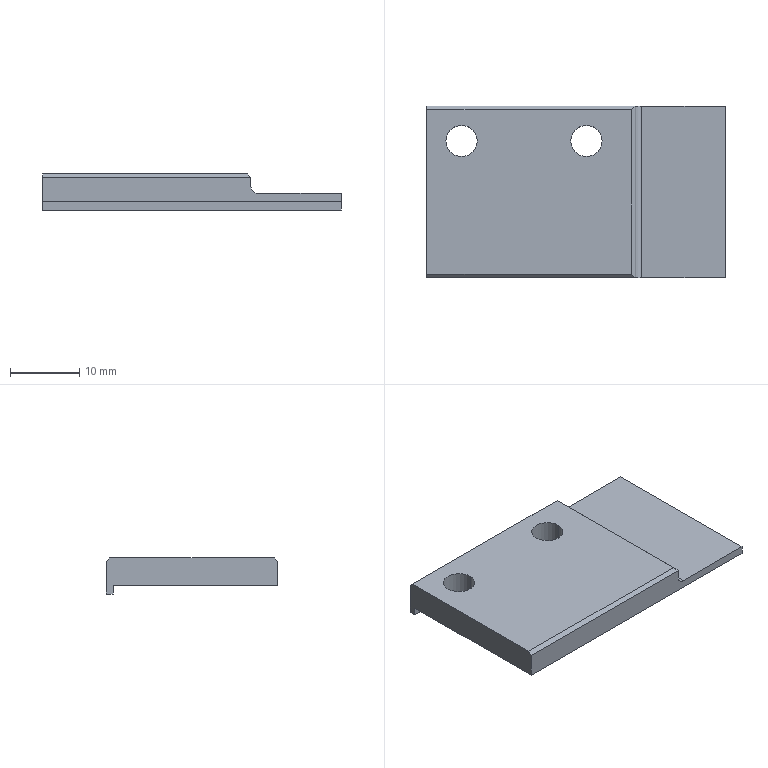Part | NX | 1 solid | 18 faces | box 43 x 24.7 x 5.2 mm | volume 3268 mm3 | plane 13 | cylinder 5 | commonest cylinder face diameters 4.5 x4 2 x1
STEP:
#1=CARTESIAN_POINT('',(0.,0.,-0.2));
#2=VERTEX_POINT('',#1);
#3=CARTESIAN_POINT('',(0.,-1.,-0.2));
#4=VERTEX_POINT('',#3);
#5=CARTESIAN_POINT('',(0.,0.,-0.2));
#6=DIRECTION('',(0.,-1.,0.));
#7=VECTOR('',#6,1000.);
#8=LINE('',#5,#7);
#9=EDGE_CURVE('',#2,#4,#8,.T.);
#10=ORIENTED_EDGE('',*,*,#9,.F.);
#11=CARTESIAN_POINT('',(43.,0.,-0.2));
#12=VERTEX_POINT('',#11);
#13=CARTESIAN_POINT('',(0.,0.,-0.2));
#14=DIRECTION('',(1.,0.,0.));
#15=VECTOR('',#14,1000.);
#16=LINE('',#13,#15);
#17=EDGE_CURVE('',#2,#12,#16,.T.);
#18=ORIENTED_EDGE('',*,*,#17,.T.);
#19=CARTESIAN_POINT('',(43.,-1.,-0.2));
#20=VERTEX_POINT('',#19);
#21=CARTESIAN_POINT('',(43.,0.,-0.2));
#22=DIRECTION('',(0.,1.,0.));
#23=VECTOR('',#22,1000.);
#24=LINE('',#21,#23);
#25=EDGE_CURVE('',#20,#12,#24,.T.);
#26=ORIENTED_EDGE('',*,*,#25,.F.);
#27=CARTESIAN_POINT('',(0.,-1.,-0.2));
#28=DIRECTION('',(-1.,0.,0.));
#29=VECTOR('',#28,1000.);
#30=LINE('',#27,#29);
#31=EDGE_CURVE('',#20,#4,#30,.T.);
#32=ORIENTED_EDGE('',*,*,#31,.T.);
#33=EDGE_LOOP('',(#10,#18,#26,#32));
#34=FACE_BOUND('',#33,.T.);
#35=CARTESIAN_POINT('',(0.,0.,-0.2));
#36=DIRECTION('',(0.,0.,1.));
#37=DIRECTION('',(1.,0.,0.));
#38=AXIS2_PLACEMENT_3D('',#35,#36,#37);
#39=PLANE('',#38);
#40=ADVANCED_FACE('',(#34),#39,.F.);
#41=ORIENTED_EDGE('',*,*,#9,.T.);
#42=CARTESIAN_POINT('',(0.,-1.,1.));
#43=VERTEX_POINT('',#42);
#44=CARTESIAN_POINT('',(0.,-1.,0.));
#45=DIRECTION('',(0.,0.,-1.));
#46=VECTOR('',#45,1000.);
#47=LINE('',#44,#46);
#48=EDGE_CURVE('',#43,#4,#47,.T.);
#49=ORIENTED_EDGE('',*,*,#48,.F.);
#50=CARTESIAN_POINT('',(0.,-24.7,1.));
#51=VERTEX_POINT('',#50);
#52=CARTESIAN_POINT('',(0.,0.,1.));
#53=DIRECTION('',(0.,-1.,0.));
#54=VECTOR('',#53,1000.);
#55=LINE('',#52,#54);
#56=EDGE_CURVE('',#43,#51,#55,.T.);
#57=ORIENTED_EDGE('',*,*,#56,.T.);
#58=CARTESIAN_POINT('',(0.,-24.7,4.5));
#59=VERTEX_POINT('',#58);
#60=CARTESIAN_POINT('',(0.,-24.7,0.));
#61=DIRECTION('',(0.,0.,-1.));
#62=VECTOR('',#61,1000.);
#63=LINE('',#60,#62);
#64=EDGE_CURVE('',#59,#51,#63,.T.);
#65=ORIENTED_EDGE('',*,*,#64,.F.);
#66=CARTESIAN_POINT('',(0.,-24.2,5.));
#67=VERTEX_POINT('',#66);
#68=CARTESIAN_POINT('',(0.,-29.2,0.));
#69=DIRECTION('',(0.,0.7071,0.7071));
#70=VECTOR('',#69,1000.);
#71=LINE('',#68,#70);
#72=EDGE_CURVE('',#59,#67,#71,.T.);
#73=ORIENTED_EDGE('',*,*,#72,.T.);
#74=CARTESIAN_POINT('',(0.,-0.5,5.));
#75=VERTEX_POINT('',#74);
#76=CARTESIAN_POINT('',(0.,0.,5.));
#77=DIRECTION('',(0.,-1.,0.));
#78=VECTOR('',#77,1000.);
#79=LINE('',#76,#78);
#80=EDGE_CURVE('',#75,#67,#79,.T.);
#81=ORIENTED_EDGE('',*,*,#80,.F.);
#82=CARTESIAN_POINT('',(0.,0.,4.5));
#83=VERTEX_POINT('',#82);
#84=CARTESIAN_POINT('',(0.,4.5,0.));
#85=DIRECTION('',(0.,-0.7071,0.7071));
#86=VECTOR('',#85,1000.);
#87=LINE('',#84,#86);
#88=EDGE_CURVE('',#83,#75,#87,.T.);
#89=ORIENTED_EDGE('',*,*,#88,.F.);
#90=CARTESIAN_POINT('',(0.,0.,0.));
#91=DIRECTION('',(0.,0.,1.));
#92=VECTOR('',#91,1000.);
#93=LINE('',#90,#92);
#94=EDGE_CURVE('',#2,#83,#93,.T.);
#95=ORIENTED_EDGE('',*,*,#94,.F.);
#96=EDGE_LOOP('',(#41,#49,#57,#65,#73,#81,#89,#95));
#97=FACE_BOUND('',#96,.T.);
#98=CARTESIAN_POINT('',(0.,0.,0.));
#99=DIRECTION('',(-1.,0.,0.));
#100=DIRECTION('',(0.,0.,1.));
#101=AXIS2_PLACEMENT_3D('',#98,#99,#100);
#102=PLANE('',#101);
#103=ADVANCED_FACE('',(#97),#102,.T.);
#104=CARTESIAN_POINT('',(31.,0.,2.2));
#105=VERTEX_POINT('',#104);
#106=CARTESIAN_POINT('',(43.,0.,2.2));
#107=VERTEX_POINT('',#106);
#108=CARTESIAN_POINT('',(0.,0.,2.2));
#109=DIRECTION('',(1.,0.,0.));
#110=VECTOR('',#109,1000.);
#111=LINE('',#108,#110);
#112=EDGE_CURVE('',#105,#107,#111,.T.);
#113=ORIENTED_EDGE('',*,*,#112,.T.);
#114=CARTESIAN_POINT('',(43.,0.,0.));
#115=DIRECTION('',(0.,0.,-1.));
#116=VECTOR('',#115,1000.);
#117=LINE('',#114,#116);
#118=EDGE_CURVE('',#107,#12,#117,.T.);
#119=ORIENTED_EDGE('',*,*,#118,.T.);
#120=ORIENTED_EDGE('',*,*,#17,.F.);
#121=ORIENTED_EDGE('',*,*,#94,.T.);
#122=CARTESIAN_POINT('',(30.,0.,4.5));
#123=VERTEX_POINT('',#122);
#124=CARTESIAN_POINT('',(0.,0.,4.5));
#125=DIRECTION('',(1.,0.,0.));
#126=VECTOR('',#125,1000.);
#127=LINE('',#124,#126);
#128=EDGE_CURVE('',#83,#123,#127,.T.);
#129=ORIENTED_EDGE('',*,*,#128,.T.);
#130=CARTESIAN_POINT('',(30.,0.,3.2));
#131=VERTEX_POINT('',#130);
#132=CARTESIAN_POINT('',(30.,0.,0.));
#133=DIRECTION('',(0.,0.,1.));
#134=VECTOR('',#133,1000.);
#135=LINE('',#132,#134);
#136=EDGE_CURVE('',#131,#123,#135,.T.);
#137=ORIENTED_EDGE('',*,*,#136,.F.);
#138=CARTESIAN_POINT('',(31.,0.,3.2));
#139=DIRECTION('',(0.,1.,0.));
#140=DIRECTION('',(1.,0.,0.));
#141=AXIS2_PLACEMENT_3D('',#138,#139,#140);
#142=CIRCLE('',#141,1.);
#143=EDGE_CURVE('',#105,#131,#142,.T.);
#144=ORIENTED_EDGE('',*,*,#143,.F.);
#145=EDGE_LOOP('',(#113,#119,#120,#121,#129,#137,#144));
#146=FACE_BOUND('',#145,.T.);
#147=CARTESIAN_POINT('',(43.,0.,0.));
#148=DIRECTION('',(0.,1.,0.));
#149=DIRECTION('',(1.,0.,0.));
#150=AXIS2_PLACEMENT_3D('',#147,#148,#149);
#151=PLANE('',#150);
#152=ADVANCED_FACE('',(#146),#151,.T.);
#153=CARTESIAN_POINT('',(31.,-24.7,2.2));
#154=VERTEX_POINT('',#153);
#155=CARTESIAN_POINT('',(31.,0.,2.2));
#156=DIRECTION('',(0.,1.,0.));
#157=VECTOR('',#156,1000.);
#158=LINE('',#155,#157);
#159=EDGE_CURVE('',#154,#105,#158,.T.);
#160=ORIENTED_EDGE('',*,*,#159,.F.);
#161=CARTESIAN_POINT('',(43.,-24.7,2.2));
#162=VERTEX_POINT('',#161);
#163=CARTESIAN_POINT('',(0.,-24.7,2.2));
#164=DIRECTION('',(-1.,0.,0.));
#165=VECTOR('',#164,1000.);
#166=LINE('',#163,#165);
#167=EDGE_CURVE('',#162,#154,#166,.T.);
#168=ORIENTED_EDGE('',*,*,#167,.F.);
#169=CARTESIAN_POINT('',(43.,0.,2.2));
#170=DIRECTION('',(0.,-1.,0.));
#171=VECTOR('',#170,1000.);
#172=LINE('',#169,#171);
#173=EDGE_CURVE('',#107,#162,#172,.T.);
#174=ORIENTED_EDGE('',*,*,#173,.F.);
#175=ORIENTED_EDGE('',*,*,#112,.F.);
#176=EDGE_LOOP('',(#160,#168,#174,#175));
#177=FACE_BOUND('',#176,.T.);
#178=CARTESIAN_POINT('',(0.,0.,2.2));
#179=DIRECTION('',(0.,0.,1.));
#180=DIRECTION('',(1.,0.,0.));
#181=AXIS2_PLACEMENT_3D('',#178,#179,#180);
#182=PLANE('',#181);
#183=ADVANCED_FACE('',(#177),#182,.T.);
#184=CARTESIAN_POINT('',(30.,-24.7,4.5));
#185=VERTEX_POINT('',#184);
#186=CARTESIAN_POINT('',(30.,0.,4.5));
#187=DIRECTION('',(0.,1.,0.));
#188=VECTOR('',#187,1000.);
#189=LINE('',#186,#188);
#190=EDGE_CURVE('',#185,#123,#189,.T.);
#191=ORIENTED_EDGE('',*,*,#190,.T.);
#192=CARTESIAN_POINT('',(29.5,-0.5,5.));
#193=VERTEX_POINT('',#192);
#194=CARTESIAN_POINT('',(34.5,4.5,0.));
#195=DIRECTION('',(0.5774,0.5774,-0.5774));
#196=VECTOR('',#195,1000.);
#197=LINE('',#194,#196);
#198=EDGE_CURVE('',#193,#123,#197,.T.);
#199=ORIENTED_EDGE('',*,*,#198,.F.);
#200=CARTESIAN_POINT('',(29.5,-24.2,5.));
#201=VERTEX_POINT('',#200);
#202=CARTESIAN_POINT('',(29.5,0.,5.));
#203=DIRECTION('',(0.,1.,0.));
#204=VECTOR('',#203,1000.);
#205=LINE('',#202,#204);
#206=EDGE_CURVE('',#201,#193,#205,.T.);
#207=ORIENTED_EDGE('',*,*,#206,.F.);
#208=CARTESIAN_POINT('',(34.5,-29.2,0.));
#209=DIRECTION('',(0.5774,-0.5774,-0.5774));
#210=VECTOR('',#209,1000.);
#211=LINE('',#208,#210);
#212=EDGE_CURVE('',#201,#185,#211,.T.);
#213=ORIENTED_EDGE('',*,*,#212,.T.);
#214=EDGE_LOOP('',(#191,#199,#207,#213));
#215=FACE_BOUND('',#214,.T.);
#216=CARTESIAN_POINT('',(29.75,-12.35,4.75));
#217=DIRECTION('',(-0.7071,0.,-0.7071));
#218=DIRECTION('',(-0.7071,0.,0.7071));
#219=AXIS2_PLACEMENT_3D('',#216,#217,#218);
#220=PLANE('',#219);
#221=ADVANCED_FACE('',(#215),#220,.F.);
#222=CARTESIAN_POINT('',(30.,-24.7,3.2));
#223=VERTEX_POINT('',#222);
#224=CARTESIAN_POINT('',(30.,-24.7,0.));
#225=DIRECTION('',(0.,0.,-1.));
#226=VECTOR('',#225,1000.);
#227=LINE('',#224,#226);
#228=EDGE_CURVE('',#185,#223,#227,.T.);
#229=ORIENTED_EDGE('',*,*,#228,.F.);
#230=CARTESIAN_POINT('',(0.,-24.7,4.5));
#231=DIRECTION('',(1.,0.,0.));
#232=VECTOR('',#231,1000.);
#233=LINE('',#230,#232);
#234=EDGE_CURVE('',#59,#185,#233,.T.);
#235=ORIENTED_EDGE('',*,*,#234,.F.);
#236=ORIENTED_EDGE('',*,*,#64,.T.);
#237=CARTESIAN_POINT('',(43.,-24.7,1.));
#238=VERTEX_POINT('',#237);
#239=CARTESIAN_POINT('',(0.,-24.7,1.));
#240=DIRECTION('',(-1.,0.,0.));
#241=VECTOR('',#240,1000.);
#242=LINE('',#239,#241);
#243=EDGE_CURVE('',#238,#51,#242,.T.);
#244=ORIENTED_EDGE('',*,*,#243,.F.);
#245=CARTESIAN_POINT('',(43.,-24.7,0.));
#246=DIRECTION('',(0.,0.,1.));
#247=VECTOR('',#246,1000.);
#248=LINE('',#245,#247);
#249=EDGE_CURVE('',#238,#162,#248,.T.);
#250=ORIENTED_EDGE('',*,*,#249,.T.);
#251=ORIENTED_EDGE('',*,*,#167,.T.);
#252=CARTESIAN_POINT('',(31.,-24.7,3.2));
#253=DIRECTION('',(0.,1.,0.));
#254=DIRECTION('',(1.,0.,0.));
#255=AXIS2_PLACEMENT_3D('',#252,#253,#254);
#256=CIRCLE('',#255,1.);
#257=EDGE_CURVE('',#154,#223,#256,.T.);
#258=ORIENTED_EDGE('',*,*,#257,.T.);
#259=EDGE_LOOP('',(#229,#235,#236,#244,#250,#251,#258));
#260=FACE_BOUND('',#259,.T.);
#261=CARTESIAN_POINT('',(0.,-24.7,0.));
#262=DIRECTION('',(0.,-1.,0.));
#263=DIRECTION('',(0.,0.,-1.));
#264=AXIS2_PLACEMENT_3D('',#261,#262,#263);
#265=PLANE('',#264);
#266=ADVANCED_FACE('',(#260),#265,.T.);
#267=CARTESIAN_POINT('',(30.,0.,3.2));
#268=DIRECTION('',(0.,1.,0.));
#269=VECTOR('',#268,1000.);
#270=LINE('',#267,#269);
#271=EDGE_CURVE('',#223,#131,#270,.T.);
#272=ORIENTED_EDGE('',*,*,#271,.T.);
#273=ORIENTED_EDGE('',*,*,#136,.T.);
#274=ORIENTED_EDGE('',*,*,#190,.F.);
#275=ORIENTED_EDGE('',*,*,#228,.T.);
#276=EDGE_LOOP('',(#272,#273,#274,#275));
#277=FACE_BOUND('',#276,.T.);
#278=CARTESIAN_POINT('',(30.,0.,5.));
#279=DIRECTION('',(-1.,0.,0.));
#280=DIRECTION('',(0.,0.,1.));
#281=AXIS2_PLACEMENT_3D('',#278,#279,#280);
#282=PLANE('',#281);
#283=ADVANCED_FACE('',(#277),#282,.F.);
#284=ORIENTED_EDGE('',*,*,#206,.T.);
#285=CARTESIAN_POINT('',(0.,-0.5,5.));
#286=DIRECTION('',(1.,0.,0.));
#287=VECTOR('',#286,1000.);
#288=LINE('',#285,#287);
#289=EDGE_CURVE('',#75,#193,#288,.T.);
#290=ORIENTED_EDGE('',*,*,#289,.F.);
#291=ORIENTED_EDGE('',*,*,#80,.T.);
#292=CARTESIAN_POINT('',(0.,-24.2,5.));
#293=DIRECTION('',(1.,0.,0.));
#294=VECTOR('',#293,1000.);
#295=LINE('',#292,#294);
#296=EDGE_CURVE('',#67,#201,#295,.T.);
#297=ORIENTED_EDGE('',*,*,#296,.T.);
#298=EDGE_LOOP('',(#284,#290,#291,#297));
#299=FACE_BOUND('',#298,.T.);
#300=CARTESIAN_POINT('',(20.75,-5.,5.));
#301=VERTEX_POINT('',#300);
#302=CARTESIAN_POINT('',(25.25,-5.,5.));
#303=VERTEX_POINT('',#302);
#304=CARTESIAN_POINT('',(23.,-5.,5.));
#305=DIRECTION('',(0.,0.,-1.));
#306=DIRECTION('',(-1.,0.,0.));
#307=AXIS2_PLACEMENT_3D('',#304,#305,#306);
#308=CIRCLE('',#307,2.25);
#309=EDGE_CURVE('',#301,#303,#308,.T.);
#310=ORIENTED_EDGE('',*,*,#309,.T.);
#311=CARTESIAN_POINT('',(23.,-5.,5.));
#312=DIRECTION('',(0.,0.,-1.));
#313=DIRECTION('',(-1.,0.,0.));
#314=AXIS2_PLACEMENT_3D('',#311,#312,#313);
#315=CIRCLE('',#314,2.25);
#316=EDGE_CURVE('',#303,#301,#315,.T.);
#317=ORIENTED_EDGE('',*,*,#316,.T.);
#318=EDGE_LOOP('',(#310,#317));
#319=FACE_BOUND('',#318,.T.);
#320=CARTESIAN_POINT('',(7.25,-5.,5.));
#321=VERTEX_POINT('',#320);
#322=CARTESIAN_POINT('',(2.75,-5.,5.));
#323=VERTEX_POINT('',#322);
#324=CARTESIAN_POINT('',(5.,-5.,5.));
#325=DIRECTION('',(0.,0.,-1.));
#326=DIRECTION('',(-1.,0.,0.));
#327=AXIS2_PLACEMENT_3D('',#324,#325,#326);
#328=CIRCLE('',#327,2.25);
#329=EDGE_CURVE('',#321,#323,#328,.T.);
#330=ORIENTED_EDGE('',*,*,#329,.T.);
#331=CARTESIAN_POINT('',(5.,-5.,5.));
#332=DIRECTION('',(0.,0.,-1.));
#333=DIRECTION('',(-1.,0.,0.));
#334=AXIS2_PLACEMENT_3D('',#331,#332,#333);
#335=CIRCLE('',#334,2.25);
#336=EDGE_CURVE('',#323,#321,#335,.T.);
#337=ORIENTED_EDGE('',*,*,#336,.T.);
#338=EDGE_LOOP('',(#330,#337));
#339=FACE_BOUND('',#338,.T.);
#340=CARTESIAN_POINT('',(0.,0.,5.));
#341=DIRECTION('',(0.,0.,1.));
#342=DIRECTION('',(1.,0.,0.));
#343=AXIS2_PLACEMENT_3D('',#340,#341,#342);
#344=PLANE('',#343);
#345=ADVANCED_FACE('',(#299,#319,#339),#344,.T.);
#346=CARTESIAN_POINT('',(20.75,-5.,1.));
#347=VERTEX_POINT('',#346);
#348=CARTESIAN_POINT('',(25.25,-5.,1.));
#349=VERTEX_POINT('',#348);
#350=CARTESIAN_POINT('',(23.,-5.,1.));
#351=DIRECTION('',(0.,0.,-1.));
#352=DIRECTION('',(-1.,0.,0.));
#353=AXIS2_PLACEMENT_3D('',#350,#351,#352);
#354=CIRCLE('',#353,2.25);
#355=EDGE_CURVE('',#347,#349,#354,.T.);
#356=ORIENTED_EDGE('',*,*,#355,.T.);
#357=CARTESIAN_POINT('',(25.25,-5.,5.));
#358=DIRECTION('',(0.,0.,-1.));
#359=VECTOR('',#358,1000.);
#360=LINE('',#357,#359);
#361=EDGE_CURVE('',#349,#303,#360,.F.);
#362=ORIENTED_EDGE('',*,*,#361,.T.);
#363=ORIENTED_EDGE('',*,*,#309,.F.);
#364=CARTESIAN_POINT('',(20.75,-5.,5.));
#365=DIRECTION('',(0.,0.,-1.));
#366=VECTOR('',#365,1000.);
#367=LINE('',#364,#366);
#368=EDGE_CURVE('',#347,#301,#367,.F.);
#369=ORIENTED_EDGE('',*,*,#368,.F.);
#370=EDGE_LOOP('',(#356,#362,#363,#369));
#371=FACE_BOUND('',#370,.T.);
#372=CARTESIAN_POINT('',(23.,-5.,5.));
#373=DIRECTION('',(0.,0.,-1.));
#374=DIRECTION('',(-1.,0.,0.));
#375=AXIS2_PLACEMENT_3D('',#372,#373,#374);
#376=CYLINDRICAL_SURFACE('',#375,2.25);
#377=ADVANCED_FACE('',(#371),#376,.F.);
#378=ORIENTED_EDGE('',*,*,#329,.F.);
#379=CARTESIAN_POINT('',(7.25,-5.,1.));
#380=VERTEX_POINT('',#379);
#381=CARTESIAN_POINT('',(7.25,-5.,5.));
#382=DIRECTION('',(0.,0.,-1.));
#383=VECTOR('',#382,1000.);
#384=LINE('',#381,#383);
#385=EDGE_CURVE('',#321,#380,#384,.T.);
#386=ORIENTED_EDGE('',*,*,#385,.T.);
#387=CARTESIAN_POINT('',(2.75,-5.,1.));
#388=VERTEX_POINT('',#387);
#389=CARTESIAN_POINT('',(5.,-5.,1.));
#390=DIRECTION('',(0.,0.,-1.));
#391=DIRECTION('',(-1.,0.,0.));
#392=AXIS2_PLACEMENT_3D('',#389,#390,#391);
#393=CIRCLE('',#392,2.25);
#394=EDGE_CURVE('',#380,#388,#393,.T.);
#395=ORIENTED_EDGE('',*,*,#394,.T.);
#396=CARTESIAN_POINT('',(2.75,-5.,5.));
#397=DIRECTION('',(0.,0.,-1.));
#398=VECTOR('',#397,1000.);
#399=LINE('',#396,#398);
#400=EDGE_CURVE('',#323,#388,#399,.T.);
#401=ORIENTED_EDGE('',*,*,#400,.F.);
#402=EDGE_LOOP('',(#378,#386,#395,#401));
#403=FACE_BOUND('',#402,.T.);
#404=CARTESIAN_POINT('',(5.,-5.,5.));
#405=DIRECTION('',(0.,0.,-1.));
#406=DIRECTION('',(-1.,0.,0.));
#407=AXIS2_PLACEMENT_3D('',#404,#405,#406);
#408=CYLINDRICAL_SURFACE('',#407,2.25);
#409=ADVANCED_FACE('',(#403),#408,.F.);
#410=ORIENTED_EDGE('',*,*,#56,.F.);
#411=CARTESIAN_POINT('',(43.,-1.,1.));
#412=VERTEX_POINT('',#411);
#413=CARTESIAN_POINT('',(0.,-1.,1.));
#414=DIRECTION('',(-1.,0.,0.));
#415=VECTOR('',#414,1000.);
#416=LINE('',#413,#415);
#417=EDGE_CURVE('',#412,#43,#416,.T.);
#418=ORIENTED_EDGE('',*,*,#417,.F.);
#419=CARTESIAN_POINT('',(43.,0.,1.));
#420=DIRECTION('',(0.,1.,0.));
#421=VECTOR('',#420,1000.);
#422=LINE('',#419,#421);
#423=EDGE_CURVE('',#238,#412,#422,.T.);
#424=ORIENTED_EDGE('',*,*,#423,.F.);
#425=ORIENTED_EDGE('',*,*,#243,.T.);
#426=EDGE_LOOP('',(#410,#418,#424,#425));
#427=FACE_BOUND('',#426,.T.);
#428=ORIENTED_EDGE('',*,*,#355,.F.);
#429=CARTESIAN_POINT('',(23.,-5.,1.));
#430=DIRECTION('',(0.,0.,-1.));
#431=DIRECTION('',(-1.,0.,0.));
#432=AXIS2_PLACEMENT_3D('',#429,#430,#431);
#433=CIRCLE('',#432,2.25);
#434=EDGE_CURVE('',#349,#347,#433,.T.);
#435=ORIENTED_EDGE('',*,*,#434,.F.);
#436=EDGE_LOOP('',(#428,#435));
#437=FACE_BOUND('',#436,.T.);
#438=CARTESIAN_POINT('',(5.,-5.,1.));
#439=DIRECTION('',(0.,0.,-1.));
#440=DIRECTION('',(-1.,0.,0.));
#441=AXIS2_PLACEMENT_3D('',#438,#439,#440);
#442=CIRCLE('',#441,2.25);
#443=EDGE_CURVE('',#388,#380,#442,.T.);
#444=ORIENTED_EDGE('',*,*,#443,.F.);
#445=ORIENTED_EDGE('',*,*,#394,.F.);
#446=EDGE_LOOP('',(#444,#445));
#447=FACE_BOUND('',#446,.T.);
#448=CARTESIAN_POINT('',(0.,-26.7,1.));
#449=DIRECTION('',(0.,0.,1.));
#450=DIRECTION('',(1.,0.,0.));
#451=AXIS2_PLACEMENT_3D('',#448,#449,#450);
#452=PLANE('',#451);
#453=ADVANCED_FACE('',(#427,#437,#447),#452,.F.);
#454=ORIENTED_EDGE('',*,*,#173,.T.);
#455=ORIENTED_EDGE('',*,*,#249,.F.);
#456=ORIENTED_EDGE('',*,*,#423,.T.);
#457=CARTESIAN_POINT('',(43.,-1.,0.));
#458=DIRECTION('',(0.,0.,-1.));
#459=VECTOR('',#458,1000.);
#460=LINE('',#457,#459);
#461=EDGE_CURVE('',#412,#20,#460,.T.);
#462=ORIENTED_EDGE('',*,*,#461,.T.);
#463=ORIENTED_EDGE('',*,*,#25,.T.);
#464=ORIENTED_EDGE('',*,*,#118,.F.);
#465=EDGE_LOOP('',(#454,#455,#456,#462,#463,#464));
#466=FACE_BOUND('',#465,.T.);
#467=CARTESIAN_POINT('',(43.,-26.7,0.));
#468=DIRECTION('',(1.,0.,0.));
#469=DIRECTION('',(0.,1.,0.));
#470=AXIS2_PLACEMENT_3D('',#467,#468,#469);
#471=PLANE('',#470);
#472=ADVANCED_FACE('',(#466),#471,.T.);
#473=ORIENTED_EDGE('',*,*,#31,.F.);
#474=ORIENTED_EDGE('',*,*,#461,.F.);
#475=ORIENTED_EDGE('',*,*,#417,.T.);
#476=ORIENTED_EDGE('',*,*,#48,.T.);
#477=EDGE_LOOP('',(#473,#474,#475,#476));
#478=FACE_BOUND('',#477,.T.);
#479=CARTESIAN_POINT('',(0.,-1.,1.));
#480=DIRECTION('',(0.,1.,0.));
#481=DIRECTION('',(1.,0.,0.));
#482=AXIS2_PLACEMENT_3D('',#479,#480,#481);
#483=PLANE('',#482);
#484=ADVANCED_FACE('',(#478),#483,.F.);
#485=ORIENTED_EDGE('',*,*,#128,.F.);
#486=ORIENTED_EDGE('',*,*,#88,.T.);
#487=ORIENTED_EDGE('',*,*,#289,.T.);
#488=ORIENTED_EDGE('',*,*,#198,.T.);
#489=EDGE_LOOP('',(#485,#486,#487,#488));
#490=FACE_BOUND('',#489,.T.);
#491=CARTESIAN_POINT('',(15.,-0.25,4.75));
#492=DIRECTION('',(0.,0.7071,0.7071));
#493=DIRECTION('',(1.,0.,0.));
#494=AXIS2_PLACEMENT_3D('',#491,#492,#493);
#495=PLANE('',#494);
#496=ADVANCED_FACE('',(#490),#495,.T.);
#497=ORIENTED_EDGE('',*,*,#234,.T.);
#498=ORIENTED_EDGE('',*,*,#212,.F.);
#499=ORIENTED_EDGE('',*,*,#296,.F.);
#500=ORIENTED_EDGE('',*,*,#72,.F.);
#501=EDGE_LOOP('',(#497,#498,#499,#500));
#502=FACE_BOUND('',#501,.T.);
#503=CARTESIAN_POINT('',(15.,-24.45,4.75));
#504=DIRECTION('',(0.,0.7071,-0.7071));
#505=DIRECTION('',(-1.,0.,0.));
#506=AXIS2_PLACEMENT_3D('',#503,#504,#505);
#507=PLANE('',#506);
#508=ADVANCED_FACE('',(#502),#507,.F.);
#509=ORIENTED_EDGE('',*,*,#159,.T.);
#510=ORIENTED_EDGE('',*,*,#143,.T.);
#511=ORIENTED_EDGE('',*,*,#271,.F.);
#512=ORIENTED_EDGE('',*,*,#257,.F.);
#513=EDGE_LOOP('',(#509,#510,#511,#512));
#514=FACE_BOUND('',#513,.T.);
#515=CARTESIAN_POINT('',(31.,0.,3.2));
#516=DIRECTION('',(0.,1.,0.));
#517=DIRECTION('',(1.,0.,0.));
#518=AXIS2_PLACEMENT_3D('',#515,#516,#517);
#519=CYLINDRICAL_SURFACE('',#518,1.);
#520=ADVANCED_FACE('',(#514),#519,.F.);
#521=ORIENTED_EDGE('',*,*,#368,.T.);
#522=ORIENTED_EDGE('',*,*,#316,.F.);
#523=ORIENTED_EDGE('',*,*,#361,.F.);
#524=ORIENTED_EDGE('',*,*,#434,.T.);
#525=EDGE_LOOP('',(#521,#522,#523,#524));
#526=FACE_BOUND('',#525,.T.);
#527=CARTESIAN_POINT('',(23.,-5.,5.));
#528=DIRECTION('',(0.,0.,-1.));
#529=DIRECTION('',(-1.,0.,0.));
#530=AXIS2_PLACEMENT_3D('',#527,#528,#529);
#531=CYLINDRICAL_SURFACE('',#530,2.25);
#532=ADVANCED_FACE('',(#526),#531,.F.);
#533=ORIENTED_EDGE('',*,*,#443,.T.);
#534=ORIENTED_EDGE('',*,*,#385,.F.);
#535=ORIENTED_EDGE('',*,*,#336,.F.);
#536=ORIENTED_EDGE('',*,*,#400,.T.);
#537=EDGE_LOOP('',(#533,#534,#535,#536));
#538=FACE_BOUND('',#537,.T.);
#539=CARTESIAN_POINT('',(5.,-5.,5.));
#540=DIRECTION('',(0.,0.,-1.));
#541=DIRECTION('',(-1.,0.,0.));
#542=AXIS2_PLACEMENT_3D('',#539,#540,#541);
#543=CYLINDRICAL_SURFACE('',#542,2.25);
#544=ADVANCED_FACE('',(#538),#543,.F.);
#545=CLOSED_SHELL('',(#40,#103,#152,#183,#221,#266,#283,#345,#377,#409,#453,#472,#484,#496,#508,#520,#532,#544));
#546=MANIFOLD_SOLID_BREP('',#545);
#547=(LENGTH_UNIT()NAMED_UNIT(*)SI_UNIT(.MILLI.,.METRE.));
#548=UNCERTAINTY_MEASURE_WITH_UNIT(LENGTH_MEASURE(0.00001),#547,'','');
#549=(NAMED_UNIT(*)PLANE_ANGLE_UNIT()SI_UNIT($,.RADIAN.));
#550=(NAMED_UNIT(*)SI_UNIT($,.STERADIAN.)SOLID_ANGLE_UNIT());
#551=(GEOMETRIC_REPRESENTATION_CONTEXT(3)GLOBAL_UNCERTAINTY_ASSIGNED_CONTEXT((#548))GLOBAL_UNIT_ASSIGNED_CONTEXT((#547,#549,#550))REPRESENTATION_CONTEXT('',''));
#552=ADVANCED_BREP_SHAPE_REPRESENTATION('',(#546),#551);